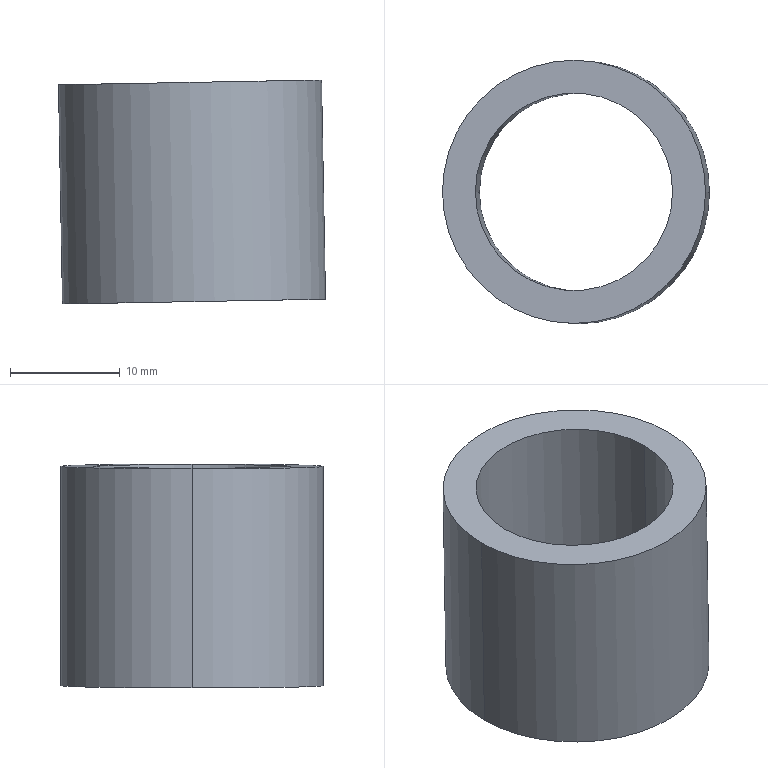Part | STEP file | 2026.6.15-Main Assembly图.sldasm-Part-5 | 1 solid | 6 faces | box 24.36 x 24 x 20.433 mm | volume 3958 mm3 | cylinder 4 | plane 2 | commonest cylinder face diameters 18 x2 24 x2
STEP:
#1=CARTESIAN_POINT('',(-908.117,668.041,3325.294));
#2=VERTEX_POINT('',#1);
#3=CARTESIAN_POINT('',(-926.114,668.041,3324.966));
#4=VERTEX_POINT('',#3);
#5=CARTESIAN_POINT('',(-917.116,668.041,3325.13));
#6=DIRECTION('',(0.01819,0.,-0.9998));
#7=DIRECTION('',(-0.9998,0.,-0.01819));
#8=AXIS2_PLACEMENT_3D('',#5,#6,#7);
#9=CIRCLE('',#8,9.);
#10=EDGE_CURVE('',#2,#4,#9,.T.);
#11=ORIENTED_EDGE('',*,*,#10,.F.);
#12=CARTESIAN_POINT('',(-907.753,668.041,3305.297));
#13=VERTEX_POINT('',#12);
#14=CARTESIAN_POINT('',(-908.499,668.041,3346.29));
#15=DIRECTION('',(0.01819,0.,-0.9998));
#16=VECTOR('',#15,1000.);
#17=LINE('',#14,#16);
#18=EDGE_CURVE('',#2,#13,#17,.T.);
#19=ORIENTED_EDGE('',*,*,#18,.T.);
#20=CARTESIAN_POINT('',(-925.75,668.041,3304.969));
#21=VERTEX_POINT('',#20);
#22=CARTESIAN_POINT('',(-916.752,668.041,3305.133));
#23=DIRECTION('',(0.01819,0.,-0.9998));
#24=DIRECTION('',(-0.9998,0.,-0.01819));
#25=AXIS2_PLACEMENT_3D('',#22,#23,#24);
#26=CIRCLE('',#25,9.);
#27=EDGE_CURVE('',#13,#21,#26,.T.);
#28=ORIENTED_EDGE('',*,*,#27,.T.);
#29=CARTESIAN_POINT('',(-926.496,668.041,3345.963));
#30=DIRECTION('',(0.01819,0.,-0.9998));
#31=VECTOR('',#30,1000.);
#32=LINE('',#29,#31);
#33=EDGE_CURVE('',#4,#21,#32,.T.);
#34=ORIENTED_EDGE('',*,*,#33,.F.);
#35=EDGE_LOOP('',(#11,#19,#28,#34));
#36=FACE_OUTER_BOUND('',#35,.T.);
#37=CARTESIAN_POINT('',(-917.498,668.041,3346.126));
#38=DIRECTION('',(0.01819,0.,-0.9998));
#39=DIRECTION('',(0.9998,0.,0.01819));
#40=AXIS2_PLACEMENT_3D('',#37,#38,#39);
#41=CYLINDRICAL_SURFACE('',#40,9.);
#42=ADVANCED_FACE('',(#36),#41,.F.);
#43=CARTESIAN_POINT('',(-928.75,668.041,3304.915));
#44=VERTEX_POINT('',#43);
#45=CARTESIAN_POINT('',(-904.754,668.041,3305.351));
#46=VERTEX_POINT('',#45);
#47=CARTESIAN_POINT('',(-916.752,668.041,3305.133));
#48=DIRECTION('',(0.01819,0.,-0.9998));
#49=DIRECTION('',(-0.9998,0.,-0.01819));
#50=AXIS2_PLACEMENT_3D('',#47,#48,#49);
#51=CIRCLE('',#50,12.);
#52=EDGE_CURVE('',#44,#46,#51,.T.);
#53=ORIENTED_EDGE('',*,*,#52,.F.);
#54=CARTESIAN_POINT('',(-929.114,668.041,3324.912));
#55=VERTEX_POINT('',#54);
#56=CARTESIAN_POINT('',(-928.75,668.041,3304.915));
#57=DIRECTION('',(0.01819,0.,-0.9998));
#58=VECTOR('',#57,1000.);
#59=LINE('',#56,#58);
#60=EDGE_CURVE('',#55,#44,#59,.T.);
#61=ORIENTED_EDGE('',*,*,#60,.F.);
#62=CARTESIAN_POINT('',(-905.118,668.041,3325.348));
#63=VERTEX_POINT('',#62);
#64=CARTESIAN_POINT('',(-917.116,668.041,3325.13));
#65=DIRECTION('',(0.01819,0.,-0.9998));
#66=DIRECTION('',(-0.9998,0.,-0.01819));
#67=AXIS2_PLACEMENT_3D('',#64,#65,#66);
#68=CIRCLE('',#67,12.);
#69=EDGE_CURVE('',#55,#63,#68,.T.);
#70=ORIENTED_EDGE('',*,*,#69,.T.);
#71=CARTESIAN_POINT('',(-904.754,668.041,3305.351));
#72=DIRECTION('',(0.01819,0.,-0.9998));
#73=VECTOR('',#72,1000.);
#74=LINE('',#71,#73);
#75=EDGE_CURVE('',#63,#46,#74,.T.);
#76=ORIENTED_EDGE('',*,*,#75,.T.);
#77=EDGE_LOOP('',(#53,#61,#70,#76));
#78=FACE_OUTER_BOUND('',#77,.T.);
#79=CARTESIAN_POINT('',(-916.752,668.041,3305.133));
#80=DIRECTION('',(-0.01819,0.,0.9998));
#81=DIRECTION('',(-0.9998,0.,-0.01819));
#82=AXIS2_PLACEMENT_3D('',#79,#80,#81);
#83=CYLINDRICAL_SURFACE('',#82,12.);
#84=ADVANCED_FACE('',(#78),#83,.T.);
#85=ORIENTED_EDGE('',*,*,#60,.T.);
#86=CARTESIAN_POINT('',(-916.752,668.041,3305.133));
#87=DIRECTION('',(0.01819,0.,-0.9998));
#88=DIRECTION('',(-0.9998,0.,-0.01819));
#89=AXIS2_PLACEMENT_3D('',#86,#87,#88);
#90=CIRCLE('',#89,12.);
#91=EDGE_CURVE('',#46,#44,#90,.T.);
#92=ORIENTED_EDGE('',*,*,#91,.F.);
#93=ORIENTED_EDGE('',*,*,#75,.F.);
#94=CARTESIAN_POINT('',(-917.116,668.041,3325.13));
#95=DIRECTION('',(0.01819,0.,-0.9998));
#96=DIRECTION('',(-0.9998,0.,-0.01819));
#97=AXIS2_PLACEMENT_3D('',#94,#95,#96);
#98=CIRCLE('',#97,12.);
#99=EDGE_CURVE('',#63,#55,#98,.T.);
#100=ORIENTED_EDGE('',*,*,#99,.T.);
#101=EDGE_LOOP('',(#85,#92,#93,#100));
#102=FACE_OUTER_BOUND('',#101,.T.);
#103=CARTESIAN_POINT('',(-916.752,668.041,3305.133));
#104=DIRECTION('',(-0.01819,0.,0.9998));
#105=DIRECTION('',(-0.9998,0.,-0.01819));
#106=AXIS2_PLACEMENT_3D('',#103,#104,#105);
#107=CYLINDRICAL_SURFACE('',#106,12.);
#108=ADVANCED_FACE('',(#102),#107,.T.);
#109=ORIENTED_EDGE('',*,*,#91,.T.);
#110=ORIENTED_EDGE('',*,*,#52,.T.);
#111=EDGE_LOOP('',(#109,#110));
#112=FACE_OUTER_BOUND('',#111,.T.);
#113=CARTESIAN_POINT('',(-916.752,668.041,3305.133));
#114=DIRECTION('',(0.01819,0.,-0.9998));
#115=DIRECTION('',(-0.9998,0.,-0.01819));
#116=AXIS2_PLACEMENT_3D('',#113,#114,#115);
#117=CIRCLE('',#116,9.);
#118=EDGE_CURVE('',#21,#13,#117,.T.);
#119=ORIENTED_EDGE('',*,*,#118,.F.);
#120=ORIENTED_EDGE('',*,*,#27,.F.);
#121=EDGE_LOOP('',(#119,#120));
#122=FACE_BOUND('',#121,.T.);
#123=CARTESIAN_POINT('',(-916.752,668.041,3305.133));
#124=DIRECTION('',(0.01819,0.,-0.9998));
#125=DIRECTION('',(0.9998,0.,0.01819));
#126=AXIS2_PLACEMENT_3D('',#123,#124,#125);
#127=PLANE('',#126);
#128=ADVANCED_FACE('',(#112,#122),#127,.T.);
#129=ORIENTED_EDGE('',*,*,#99,.F.);
#130=ORIENTED_EDGE('',*,*,#69,.F.);
#131=EDGE_LOOP('',(#129,#130));
#132=FACE_OUTER_BOUND('',#131,.T.);
#133=CARTESIAN_POINT('',(-917.116,668.041,3325.13));
#134=DIRECTION('',(0.01819,0.,-0.9998));
#135=DIRECTION('',(-0.9998,0.,-0.01819));
#136=AXIS2_PLACEMENT_3D('',#133,#134,#135);
#137=CIRCLE('',#136,9.);
#138=EDGE_CURVE('',#4,#2,#137,.T.);
#139=ORIENTED_EDGE('',*,*,#138,.T.);
#140=ORIENTED_EDGE('',*,*,#10,.T.);
#141=EDGE_LOOP('',(#139,#140));
#142=FACE_BOUND('',#141,.T.);
#143=CARTESIAN_POINT('',(-917.116,668.041,3325.13));
#144=DIRECTION('',(0.01819,0.,-0.9998));
#145=DIRECTION('',(0.9998,0.,0.01819));
#146=AXIS2_PLACEMENT_3D('',#143,#144,#145);
#147=PLANE('',#146);
#148=ADVANCED_FACE('',(#132,#142),#147,.F.);
#149=ORIENTED_EDGE('',*,*,#18,.F.);
#150=ORIENTED_EDGE('',*,*,#138,.F.);
#151=ORIENTED_EDGE('',*,*,#33,.T.);
#152=ORIENTED_EDGE('',*,*,#118,.T.);
#153=EDGE_LOOP('',(#149,#150,#151,#152));
#154=FACE_OUTER_BOUND('',#153,.T.);
#155=CARTESIAN_POINT('',(-917.498,668.041,3346.126));
#156=DIRECTION('',(0.01819,0.,-0.9998));
#157=DIRECTION('',(0.9998,0.,0.01819));
#158=AXIS2_PLACEMENT_3D('',#155,#156,#157);
#159=CYLINDRICAL_SURFACE('',#158,9.);
#160=ADVANCED_FACE('',(#154),#159,.F.);
#161=CLOSED_SHELL('',(#42,#84,#108,#128,#148,#160));
#162=MANIFOLD_SOLID_BREP('',#161);
#163=CARTESIAN_POINT('',(0.,0.,0.));
#164=DIRECTION('',(0.,0.,1.));
#165=DIRECTION('',(1.,0.,0.));
#166=AXIS2_PLACEMENT_3D('',#163,#164,#165);
#167=(LENGTH_UNIT()NAMED_UNIT(*)SI_UNIT(.MILLI.,.METRE.));
#168=UNCERTAINTY_MEASURE_WITH_UNIT(LENGTH_MEASURE(0.00001),#167,'','');
#169=(NAMED_UNIT(*)PLANE_ANGLE_UNIT()SI_UNIT($,.RADIAN.));
#170=(NAMED_UNIT(*)SI_UNIT($,.STERADIAN.)SOLID_ANGLE_UNIT());
#171=(GEOMETRIC_REPRESENTATION_CONTEXT(3)GLOBAL_UNCERTAINTY_ASSIGNED_CONTEXT((#168))GLOBAL_UNIT_ASSIGNED_CONTEXT((#167,#169,#170))REPRESENTATION_CONTEXT('',''));
#172=ADVANCED_BREP_SHAPE_REPRESENTATION('',(#162,#166),#171);